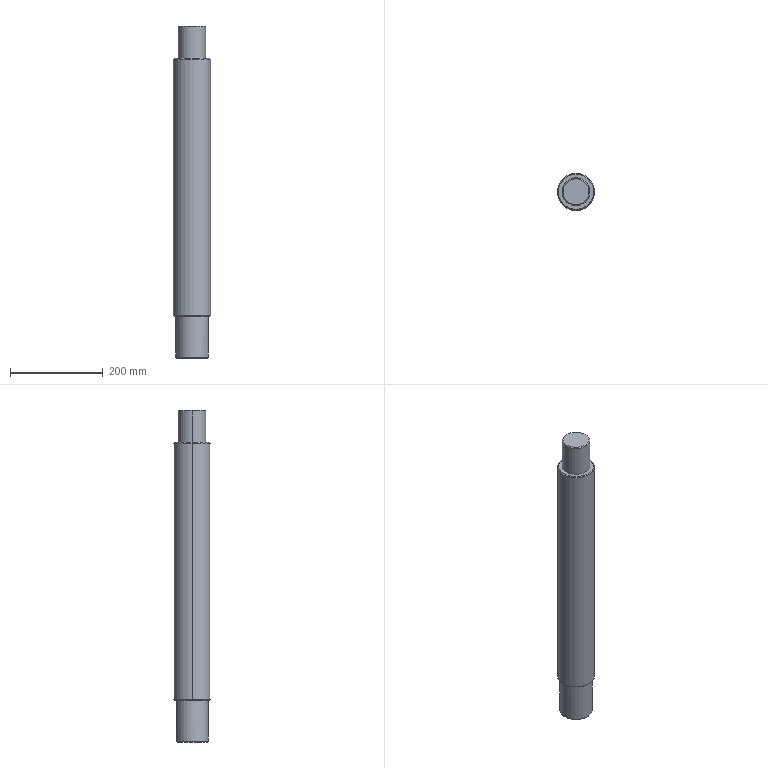Part | Creo | features CURVE 4, CUT 3, DATUM PLANE 3, CHAMFER 1, COORDINATE SYSTEM 1, PROTRUSION 1, ROUND 1 | 1 solid | 21 faces | box 80 x 80 x 717 mm | volume 3328283 mm3 | plane 7 | cylinder 7 | cone 7 | commonest cylinder face diameters 60 x2 70 x2 80 x2 20 x1
STEP:
#1=CARTESIAN_POINT('',(0.,0.,0.));
#2=DIRECTION('',(0.,0.,1.));
#3=DIRECTION('',(1.,0.,0.));
#4=AXIS2_PLACEMENT_3D('',#1,#2,#3);
#5=CARTESIAN_POINT('',(10.,31.448,0.));
#6=VERTEX_POINT('',#5);
#7=CARTESIAN_POINT('',(10.,26.541,0.));
#8=VERTEX_POINT('',#7);
#9=CARTESIAN_POINT('',(10.,31.448,0.));
#10=DIRECTION('',(0.,-1.,0.));
#11=VECTOR('',#10,4.907);
#12=LINE('',#9,#11);
#13=EDGE_CURVE('',#6,#8,#12,.T.);
#14=ORIENTED_EDGE('',*,*,#13,.T.);
#15=CARTESIAN_POINT('',(-10.,26.541,0.));
#16=VERTEX_POINT('',#15);
#17=CARTESIAN_POINT('',(10.,26.541,0.));
#18=DIRECTION('',(-1.,0.,0.));
#19=VECTOR('',#18,20.);
#20=LINE('',#17,#19);
#21=EDGE_CURVE('',#8,#16,#20,.T.);
#22=ORIENTED_EDGE('',*,*,#21,.T.);
#23=CARTESIAN_POINT('',(-10.,31.448,0.));
#24=VERTEX_POINT('',#23);
#25=CARTESIAN_POINT('',(-10.,31.448,0.));
#26=DIRECTION('',(0.,-1.,0.));
#27=VECTOR('',#26,4.907);
#28=LINE('',#25,#27);
#29=EDGE_CURVE('',#24,#16,#28,.T.);
#30=ORIENTED_EDGE('',*,*,#29,.F.);
#31=CARTESIAN_POINT('',(0.,0.,0.));
#32=DIRECTION('',(0.,0.,-1.));
#33=DIRECTION('',(0.303,0.953,0.));
#34=AXIS2_PLACEMENT_3D('',#31,#32,#33);
#35=CIRCLE('',#34,33.);
#36=EDGE_CURVE('',#6,#24,#35,.T.);
#37=ORIENTED_EDGE('',*,*,#36,.F.);
#38=EDGE_LOOP('',(#14,#22,#30,#37));
#39=FACE_OUTER_BOUND('',#38,.F.);
#40=CARTESIAN_POINT('',(0.,0.,0.));
#41=DIRECTION('',(0.,0.,1.));
#42=DIRECTION('',(1.,0.,0.));
#43=AXIS2_PLACEMENT_3D('',#40,#41,#42);
#44=PLANE('',#43);
#45=ADVANCED_FACE('',(#39),#44,.F.);
#46=CARTESIAN_POINT('',(10.,26.541,80.));
#47=VERTEX_POINT('',#46);
#48=CARTESIAN_POINT('',(10.,33.541,80.));
#49=VERTEX_POINT('',#48);
#50=CARTESIAN_POINT('',(10.,26.541,80.));
#51=DIRECTION('',(0.,1.,0.));
#52=VECTOR('',#51,7.);
#53=LINE('',#50,#52);
#54=EDGE_CURVE('',#47,#49,#53,.T.);
#55=ORIENTED_EDGE('',*,*,#54,.F.);
#56=CARTESIAN_POINT('',(10.,26.541,0.));
#57=DIRECTION('',(0.,0.,1.));
#58=VECTOR('',#57,80.);
#59=LINE('',#56,#58);
#60=EDGE_CURVE('',#8,#47,#59,.T.);
#61=ORIENTED_EDGE('',*,*,#60,.F.);
#62=ORIENTED_EDGE('',*,*,#13,.F.);
#63=CARTESIAN_POINT('',(10.,33.541,2.));
#64=VERTEX_POINT('',#63);
#65=CARTESIAN_POINT('',(10.,31.448,0.));
#66=CARTESIAN_POINT('',(10.,31.678,0.2193));
#67=CARTESIAN_POINT('',(10.,32.14,0.6599));
#68=CARTESIAN_POINT('',(10.,32.838,1.327));
#69=CARTESIAN_POINT('',(10.,33.306,1.775));
#70=B_SPLINE_CURVE_WITH_KNOTS('',3,(#65,#66,#67,#68,#69,#63),.UNSPECIFIED.,.F.,.F.,(4,1,1,4),(0.,0.3333,0.6667,1.),.UNSPECIFIED.);
#71=EDGE_CURVE('',#6,#64,#70,.T.);
#72=ORIENTED_EDGE('',*,*,#71,.T.);
#73=CARTESIAN_POINT('',(10.,33.541,80.));
#74=DIRECTION('',(0.,0.,-1.));
#75=VECTOR('',#74,78.);
#76=LINE('',#73,#75);
#77=EDGE_CURVE('',#49,#64,#76,.T.);
#78=ORIENTED_EDGE('',*,*,#77,.F.);
#79=EDGE_LOOP('',(#55,#61,#62,#72,#78));
#80=FACE_OUTER_BOUND('',#79,.F.);
#81=CARTESIAN_POINT('',(10.,33.541,0.));
#82=DIRECTION('',(1.,0.,0.));
#83=DIRECTION('',(0.,-1.,0.));
#84=AXIS2_PLACEMENT_3D('',#81,#82,#83);
#85=PLANE('',#84);
#86=ADVANCED_FACE('',(#80),#85,.F.);
#87=CARTESIAN_POINT('',(-10.,33.541,80.));
#88=VERTEX_POINT('',#87);
#89=CARTESIAN_POINT('',(-10.,26.541,80.));
#90=VERTEX_POINT('',#89);
#91=CARTESIAN_POINT('',(-10.,33.541,80.));
#92=DIRECTION('',(0.,-1.,0.));
#93=VECTOR('',#92,7.);
#94=LINE('',#91,#93);
#95=EDGE_CURVE('',#88,#90,#94,.T.);
#96=ORIENTED_EDGE('',*,*,#95,.T.);
#97=CARTESIAN_POINT('',(0.,26.541,80.));
#98=DIRECTION('',(0.,-1.,0.));
#99=DIRECTION('',(1.,0.,0.));
#100=AXIS2_PLACEMENT_3D('',#97,#98,#99);
#101=CIRCLE('',#100,10.);
#102=EDGE_CURVE('',#47,#90,#101,.T.);
#103=ORIENTED_EDGE('',*,*,#102,.F.);
#104=ORIENTED_EDGE('',*,*,#54,.T.);
#105=CARTESIAN_POINT('',(0.,35.,90.));
#106=VERTEX_POINT('',#105);
#107=CARTESIAN_POINT('',(10.,33.541,80.));
#108=CARTESIAN_POINT('',(10.,33.541,80.659));
#109=CARTESIAN_POINT('',(9.87,33.58,81.974));
#110=CARTESIAN_POINT('',(9.292,33.747,83.866));
#111=CARTESIAN_POINT('',(8.363,33.992,85.599));
#112=CARTESIAN_POINT('',(7.117,34.278,87.115));
#113=CARTESIAN_POINT('',(5.601,34.562,88.361));
#114=CARTESIAN_POINT('',(3.867,34.802,89.292));
#115=CARTESIAN_POINT('',(1.974,34.962,89.87));
#116=CARTESIAN_POINT('',(0.6588,35.,90.));
#117=CARTESIAN_POINT('',(0.,35.,90.));
#118=B_SPLINE_CURVE_WITH_KNOTS('',3,(#107,#108,#109,#110,#111,#112,#113,#114,#115,#116,#117),.UNSPECIFIED.,.F.,.F.,(4,1,1,1,1,1,1,1,4),(0.,0.125,0.25,0.375,0.5,0.625,0.75,0.875,1.),.UNSPECIFIED.);
#119=EDGE_CURVE('',#49,#106,#118,.T.);
#120=ORIENTED_EDGE('',*,*,#119,.T.);
#121=CARTESIAN_POINT('',(0.,35.,90.));
#122=CARTESIAN_POINT('',(-0.6588,35.,90.));
#123=CARTESIAN_POINT('',(-1.974,34.962,89.87));
#124=CARTESIAN_POINT('',(-3.867,34.802,89.292));
#125=CARTESIAN_POINT('',(-5.601,34.562,88.361));
#126=CARTESIAN_POINT('',(-7.117,34.279,87.115));
#127=CARTESIAN_POINT('',(-8.362,33.993,85.599));
#128=CARTESIAN_POINT('',(-9.292,33.747,83.866));
#129=CARTESIAN_POINT('',(-9.87,33.58,81.974));
#130=CARTESIAN_POINT('',(-10.,33.541,80.659));
#131=CARTESIAN_POINT('',(-10.,33.541,80.));
#132=B_SPLINE_CURVE_WITH_KNOTS('',3,(#121,#122,#123,#124,#125,#126,#127,#128,#129,#130,#131),.UNSPECIFIED.,.F.,.F.,(4,1,1,1,1,1,1,1,4),(0.,0.125,0.25,0.375,0.5,0.625,0.75,0.875,1.),.UNSPECIFIED.);
#133=EDGE_CURVE('',#106,#88,#132,.T.);
#134=ORIENTED_EDGE('',*,*,#133,.T.);
#135=EDGE_LOOP('',(#96,#103,#104,#120,#134));
#136=FACE_OUTER_BOUND('',#135,.F.);
#137=CARTESIAN_POINT('',(0.,144.288,80.));
#138=DIRECTION('',(0.,-1.,0.));
#139=DIRECTION('',(0.,0.,1.));
#140=AXIS2_PLACEMENT_3D('',#137,#138,#139);
#141=CYLINDRICAL_SURFACE('',#140,10.);
#142=ADVANCED_FACE('',(#136),#141,.F.);
#143=ORIENTED_EDGE('',*,*,#95,.F.);
#144=CARTESIAN_POINT('',(-10.,33.541,2.));
#145=VERTEX_POINT('',#144);
#146=CARTESIAN_POINT('',(-10.,33.541,80.));
#147=DIRECTION('',(0.,0.,-1.));
#148=VECTOR('',#147,78.);
#149=LINE('',#146,#148);
#150=EDGE_CURVE('',#88,#145,#149,.T.);
#151=ORIENTED_EDGE('',*,*,#150,.T.);
#152=CARTESIAN_POINT('',(-10.,33.306,1.775));
#153=CARTESIAN_POINT('',(-10.,32.838,1.327));
#154=CARTESIAN_POINT('',(-10.,32.14,0.66));
#155=CARTESIAN_POINT('',(-10.,31.679,0.2193));
#156=CARTESIAN_POINT('',(-10.,31.448,0.));
#157=B_SPLINE_CURVE_WITH_KNOTS('',3,(#144,#152,#153,#154,#155,#156),.UNSPECIFIED.,.F.,.F.,(4,1,1,4),(0.,0.3333,0.6667,1.),.UNSPECIFIED.);
#158=EDGE_CURVE('',#145,#24,#157,.T.);
#159=ORIENTED_EDGE('',*,*,#158,.T.);
#160=ORIENTED_EDGE('',*,*,#29,.T.);
#161=CARTESIAN_POINT('',(-10.,26.541,0.));
#162=DIRECTION('',(0.,0.,1.));
#163=VECTOR('',#162,80.);
#164=LINE('',#161,#163);
#165=EDGE_CURVE('',#16,#90,#164,.T.);
#166=ORIENTED_EDGE('',*,*,#165,.T.);
#167=EDGE_LOOP('',(#143,#151,#159,#160,#166));
#168=FACE_OUTER_BOUND('',#167,.F.);
#169=CARTESIAN_POINT('',(-10.,26.541,0.));
#170=DIRECTION('',(-1.,0.,0.));
#171=DIRECTION('',(0.,1.,0.));
#172=AXIS2_PLACEMENT_3D('',#169,#170,#171);
#173=PLANE('',#172);
#174=ADVANCED_FACE('',(#168),#173,.F.);
#175=CARTESIAN_POINT('',(-10.,33.541,90.));
#176=VERTEX_POINT('',#175);
#177=CARTESIAN_POINT('',(0.,0.,90.));
#178=DIRECTION('',(0.,0.,1.));
#179=DIRECTION('',(-0.2857,0.9583,0.));
#180=AXIS2_PLACEMENT_3D('',#177,#178,#179);
#181=CIRCLE('',#180,35.);
#182=EDGE_CURVE('',#176,#106,#181,.T.);
#183=ORIENTED_EDGE('',*,*,#182,.T.);
#184=ORIENTED_EDGE('',*,*,#119,.F.);
#185=ORIENTED_EDGE('',*,*,#77,.T.);
#186=CARTESIAN_POINT('',(0.,0.,2.));
#187=DIRECTION('',(0.,0.,1.));
#188=DIRECTION('',(-0.2857,0.9583,0.));
#189=AXIS2_PLACEMENT_3D('',#186,#187,#188);
#190=CIRCLE('',#189,35.);
#191=EDGE_CURVE('',#145,#64,#190,.T.);
#192=ORIENTED_EDGE('',*,*,#191,.F.);
#193=ORIENTED_EDGE('',*,*,#150,.F.);
#194=CARTESIAN_POINT('',(-10.,33.541,90.));
#195=DIRECTION('',(0.,0.,-1.));
#196=VECTOR('',#195,10.);
#197=LINE('',#194,#196);
#198=EDGE_CURVE('',#176,#88,#197,.T.);
#199=ORIENTED_EDGE('',*,*,#198,.F.);
#200=EDGE_LOOP('',(#183,#184,#185,#192,#193,#199));
#201=FACE_OUTER_BOUND('',#200,.F.);
#202=CARTESIAN_POINT('',(0.,0.,0.));
#203=DIRECTION('',(0.,0.,-1.));
#204=DIRECTION('',(-1.,0.,0.));
#205=AXIS2_PLACEMENT_3D('',#202,#203,#204);
#206=CYLINDRICAL_SURFACE('',#205,35.);
#207=ADVANCED_FACE('',(#201),#206,.T.);
#208=CARTESIAN_POINT('',(-38.,0.,90.));
#209=VERTEX_POINT('',#208);
#210=CARTESIAN_POINT('',(38.,0.,90.));
#211=VERTEX_POINT('',#210);
#212=CARTESIAN_POINT('',(0.,0.,90.));
#213=DIRECTION('',(0.,0.,1.));
#214=DIRECTION('',(-1.,0.,0.));
#215=AXIS2_PLACEMENT_3D('',#212,#213,#214);
#216=CIRCLE('',#215,38.);
#217=EDGE_CURVE('',#209,#211,#216,.T.);
#218=ORIENTED_EDGE('',*,*,#217,.T.);
#219=CARTESIAN_POINT('',(0.,0.,90.));
#220=DIRECTION('',(0.,0.,1.));
#221=DIRECTION('',(1.,0.,0.));
#222=AXIS2_PLACEMENT_3D('',#219,#220,#221);
#223=CIRCLE('',#222,38.);
#224=EDGE_CURVE('',#211,#209,#223,.T.);
#225=ORIENTED_EDGE('',*,*,#224,.T.);
#226=EDGE_LOOP('',(#218,#225));
#227=FACE_OUTER_BOUND('',#226,.F.);
#228=ORIENTED_EDGE('',*,*,#182,.F.);
#229=CARTESIAN_POINT('',(0.,0.,90.));
#230=DIRECTION('',(0.,0.,1.));
#231=DIRECTION('',(0.,1.,0.));
#232=AXIS2_PLACEMENT_3D('',#229,#230,#231);
#233=CIRCLE('',#232,35.);
#234=EDGE_CURVE('',#106,#176,#233,.T.);
#235=ORIENTED_EDGE('',*,*,#234,.F.);
#236=EDGE_LOOP('',(#228,#235));
#237=FACE_BOUND('',#236,.F.);
#238=CARTESIAN_POINT('',(0.,0.,90.));
#239=DIRECTION('',(0.,0.,-1.));
#240=DIRECTION('',(-1.,0.,0.));
#241=AXIS2_PLACEMENT_3D('',#238,#239,#240);
#242=PLANE('',#241);
#243=ADVANCED_FACE('',(#227,#237),#242,.T.);
#244=CARTESIAN_POINT('',(-40.,0.,92.));
#245=VERTEX_POINT('',#244);
#246=CARTESIAN_POINT('',(40.,0.,92.));
#247=VERTEX_POINT('',#246);
#248=CARTESIAN_POINT('',(0.,0.,92.));
#249=DIRECTION('',(0.,0.,1.));
#250=DIRECTION('',(-1.,0.,0.));
#251=AXIS2_PLACEMENT_3D('',#248,#249,#250);
#252=CIRCLE('',#251,40.);
#253=EDGE_CURVE('',#245,#247,#252,.T.);
#254=ORIENTED_EDGE('',*,*,#253,.T.);
#255=CARTESIAN_POINT('',(40.,0.000000005,92.));
#256=DIRECTION('',(-0.7071,0.,-0.7071));
#257=VECTOR('',#256,2.828);
#258=LINE('',#255,#257);
#259=EDGE_CURVE('',#247,#211,#258,.T.);
#260=ORIENTED_EDGE('',*,*,#259,.T.);
#261=ORIENTED_EDGE('',*,*,#217,.F.);
#262=CARTESIAN_POINT('',(-40.,-0.000000005,92.));
#263=DIRECTION('',(0.7071,0.,-0.7071));
#264=VECTOR('',#263,2.828);
#265=LINE('',#262,#264);
#266=EDGE_CURVE('',#245,#209,#265,.T.);
#267=ORIENTED_EDGE('',*,*,#266,.F.);
#268=EDGE_LOOP('',(#254,#260,#261,#267));
#269=FACE_OUTER_BOUND('',#268,.F.);
#270=CARTESIAN_POINT('',(0.,0.,91.));
#271=DIRECTION('',(0.,0.,1.));
#272=DIRECTION('',(0.,-1.,0.));
#273=AXIS2_PLACEMENT_3D('',#270,#271,#272);
#274=CONICAL_SURFACE('',#273,39.,45.);
#275=ADVANCED_FACE('',(#269),#274,.T.);
#276=CARTESIAN_POINT('',(40.,0.,645.));
#277=VERTEX_POINT('',#276);
#278=CARTESIAN_POINT('',(-40.,0.,645.));
#279=VERTEX_POINT('',#278);
#280=CARTESIAN_POINT('',(0.,0.,645.));
#281=DIRECTION('',(0.,0.,-1.));
#282=DIRECTION('',(1.,0.,0.));
#283=AXIS2_PLACEMENT_3D('',#280,#281,#282);
#284=CIRCLE('',#283,40.);
#285=EDGE_CURVE('',#277,#279,#284,.T.);
#286=ORIENTED_EDGE('',*,*,#285,.F.);
#287=CARTESIAN_POINT('',(40.,0.000000005,92.));
#288=DIRECTION('',(0.,0.,1.));
#289=VECTOR('',#288,553.);
#290=LINE('',#287,#289);
#291=EDGE_CURVE('',#247,#277,#290,.T.);
#292=ORIENTED_EDGE('',*,*,#291,.F.);
#293=ORIENTED_EDGE('',*,*,#253,.F.);
#294=CARTESIAN_POINT('',(-40.,-0.000000005,92.));
#295=DIRECTION('',(0.,0.,1.));
#296=VECTOR('',#295,553.);
#297=LINE('',#294,#296);
#298=EDGE_CURVE('',#245,#279,#297,.T.);
#299=ORIENTED_EDGE('',*,*,#298,.T.);
#300=EDGE_LOOP('',(#286,#292,#293,#299));
#301=FACE_OUTER_BOUND('',#300,.F.);
#302=CARTESIAN_POINT('',(0.,0.,0.));
#303=DIRECTION('',(0.,0.,1.));
#304=DIRECTION('',(1.,0.,0.));
#305=AXIS2_PLACEMENT_3D('',#302,#303,#304);
#306=CYLINDRICAL_SURFACE('',#305,40.);
#307=ADVANCED_FACE('',(#301),#306,.T.);
#308=ORIENTED_EDGE('',*,*,#285,.T.);
#309=CARTESIAN_POINT('',(-38.,0.,647.));
#310=VERTEX_POINT('',#309);
#311=CARTESIAN_POINT('',(-40.,-0.000000005,645.));
#312=DIRECTION('',(0.7071,0.,0.7071));
#313=VECTOR('',#312,2.828);
#314=LINE('',#311,#313);
#315=EDGE_CURVE('',#279,#310,#314,.T.);
#316=ORIENTED_EDGE('',*,*,#315,.T.);
#317=CARTESIAN_POINT('',(38.,0.,647.));
#318=VERTEX_POINT('',#317);
#319=CARTESIAN_POINT('',(0.,0.,647.));
#320=DIRECTION('',(0.,0.,-1.));
#321=DIRECTION('',(1.,0.,0.));
#322=AXIS2_PLACEMENT_3D('',#319,#320,#321);
#323=CIRCLE('',#322,38.);
#324=EDGE_CURVE('',#318,#310,#323,.T.);
#325=ORIENTED_EDGE('',*,*,#324,.F.);
#326=CARTESIAN_POINT('',(40.,0.000000005,645.));
#327=DIRECTION('',(-0.7071,0.,0.7071));
#328=VECTOR('',#327,2.828);
#329=LINE('',#326,#328);
#330=EDGE_CURVE('',#277,#318,#329,.T.);
#331=ORIENTED_EDGE('',*,*,#330,.F.);
#332=EDGE_LOOP('',(#308,#316,#325,#331));
#333=FACE_OUTER_BOUND('',#332,.F.);
#334=CARTESIAN_POINT('',(0.,0.,646.));
#335=DIRECTION('',(0.,0.,-1.));
#336=DIRECTION('',(0.,-1.,0.));
#337=AXIS2_PLACEMENT_3D('',#334,#335,#336);
#338=CONICAL_SURFACE('',#337,39.,45.);
#339=ADVANCED_FACE('',(#333),#338,.T.);
#340=CARTESIAN_POINT('',(0.,0.,645.));
#341=DIRECTION('',(0.,0.,-1.));
#342=DIRECTION('',(-1.,0.,0.));
#343=AXIS2_PLACEMENT_3D('',#340,#341,#342);
#344=CIRCLE('',#343,40.);
#345=EDGE_CURVE('',#279,#277,#344,.T.);
#346=ORIENTED_EDGE('',*,*,#345,.T.);
#347=ORIENTED_EDGE('',*,*,#330,.T.);
#348=CARTESIAN_POINT('',(0.,0.,647.));
#349=DIRECTION('',(0.,0.,-1.));
#350=DIRECTION('',(-1.,0.,0.));
#351=AXIS2_PLACEMENT_3D('',#348,#349,#350);
#352=CIRCLE('',#351,38.);
#353=EDGE_CURVE('',#310,#318,#352,.T.);
#354=ORIENTED_EDGE('',*,*,#353,.F.);
#355=ORIENTED_EDGE('',*,*,#315,.F.);
#356=EDGE_LOOP('',(#346,#347,#354,#355));
#357=FACE_OUTER_BOUND('',#356,.F.);
#358=CARTESIAN_POINT('',(0.,0.,646.));
#359=DIRECTION('',(0.,0.,-1.));
#360=DIRECTION('',(0.,-1.,0.));
#361=AXIS2_PLACEMENT_3D('',#358,#359,#360);
#362=CONICAL_SURFACE('',#361,39.,45.);
#363=ADVANCED_FACE('',(#357),#362,.T.);
#364=ORIENTED_EDGE('',*,*,#345,.F.);
#365=ORIENTED_EDGE('',*,*,#298,.F.);
#366=CARTESIAN_POINT('',(0.,0.,92.));
#367=DIRECTION('',(0.,0.,1.));
#368=DIRECTION('',(1.,0.,0.));
#369=AXIS2_PLACEMENT_3D('',#366,#367,#368);
#370=CIRCLE('',#369,40.);
#371=EDGE_CURVE('',#247,#245,#370,.T.);
#372=ORIENTED_EDGE('',*,*,#371,.F.);
#373=ORIENTED_EDGE('',*,*,#291,.T.);
#374=EDGE_LOOP('',(#364,#365,#372,#373));
#375=FACE_OUTER_BOUND('',#374,.F.);
#376=CARTESIAN_POINT('',(0.,0.,0.));
#377=DIRECTION('',(0.,0.,1.));
#378=DIRECTION('',(1.,0.,0.));
#379=AXIS2_PLACEMENT_3D('',#376,#377,#378);
#380=CYLINDRICAL_SURFACE('',#379,40.);
#381=ADVANCED_FACE('',(#375),#380,.T.);
#382=ORIENTED_EDGE('',*,*,#371,.T.);
#383=ORIENTED_EDGE('',*,*,#266,.T.);
#384=ORIENTED_EDGE('',*,*,#224,.F.);
#385=ORIENTED_EDGE('',*,*,#259,.F.);
#386=EDGE_LOOP('',(#382,#383,#384,#385));
#387=FACE_OUTER_BOUND('',#386,.F.);
#388=CARTESIAN_POINT('',(0.,0.,91.));
#389=DIRECTION('',(0.,0.,1.));
#390=DIRECTION('',(0.,-1.,0.));
#391=AXIS2_PLACEMENT_3D('',#388,#389,#390);
#392=CONICAL_SURFACE('',#391,39.,45.);
#393=ADVANCED_FACE('',(#387),#392,.T.);
#394=ORIENTED_EDGE('',*,*,#324,.T.);
#395=ORIENTED_EDGE('',*,*,#353,.T.);
#396=EDGE_LOOP('',(#394,#395));
#397=FACE_OUTER_BOUND('',#396,.F.);
#398=CARTESIAN_POINT('',(30.,0.,647.));
#399=VERTEX_POINT('',#398);
#400=CARTESIAN_POINT('',(-30.,0.,647.));
#401=VERTEX_POINT('',#400);
#402=CARTESIAN_POINT('',(0.,0.,647.));
#403=DIRECTION('',(0.,0.,-1.));
#404=DIRECTION('',(1.,0.,0.));
#405=AXIS2_PLACEMENT_3D('',#402,#403,#404);
#406=CIRCLE('',#405,30.);
#407=EDGE_CURVE('',#399,#401,#406,.T.);
#408=ORIENTED_EDGE('',*,*,#407,.F.);
#409=CARTESIAN_POINT('',(0.,0.,647.));
#410=DIRECTION('',(0.,0.,-1.));
#411=DIRECTION('',(-1.,0.,0.));
#412=AXIS2_PLACEMENT_3D('',#409,#410,#411);
#413=CIRCLE('',#412,30.);
#414=EDGE_CURVE('',#401,#399,#413,.T.);
#415=ORIENTED_EDGE('',*,*,#414,.F.);
#416=EDGE_LOOP('',(#408,#415));
#417=FACE_BOUND('',#416,.F.);
#418=CARTESIAN_POINT('',(0.,0.,647.));
#419=DIRECTION('',(0.,0.,1.));
#420=DIRECTION('',(1.,0.,0.));
#421=AXIS2_PLACEMENT_3D('',#418,#419,#420);
#422=PLANE('',#421);
#423=ADVANCED_FACE('',(#397,#417),#422,.T.);
#424=CARTESIAN_POINT('',(-30.,0.,715.));
#425=VERTEX_POINT('',#424);
#426=CARTESIAN_POINT('',(30.,0.,715.));
#427=VERTEX_POINT('',#426);
#428=CARTESIAN_POINT('',(0.,0.,715.));
#429=DIRECTION('',(0.,0.,1.));
#430=DIRECTION('',(-1.,0.,0.));
#431=AXIS2_PLACEMENT_3D('',#428,#429,#430);
#432=CIRCLE('',#431,30.);
#433=EDGE_CURVE('',#425,#427,#432,.T.);
#434=ORIENTED_EDGE('',*,*,#433,.T.);
#435=CARTESIAN_POINT('',(30.,-0.00000018,715.));
#436=DIRECTION('',(0.000000001,0.000000003,-1.));
#437=VECTOR('',#436,68.);
#438=LINE('',#435,#437);
#439=EDGE_CURVE('',#427,#399,#438,.T.);
#440=ORIENTED_EDGE('',*,*,#439,.T.);
#441=ORIENTED_EDGE('',*,*,#407,.T.);
#442=CARTESIAN_POINT('',(-30.,0.00000018,715.));
#443=DIRECTION('',(-0.000000001,-0.000000003,-1.));
#444=VECTOR('',#443,68.);
#445=LINE('',#442,#444);
#446=EDGE_CURVE('',#425,#401,#445,.T.);
#447=ORIENTED_EDGE('',*,*,#446,.F.);
#448=EDGE_LOOP('',(#434,#440,#441,#447));
#449=FACE_OUTER_BOUND('',#448,.F.);
#450=CARTESIAN_POINT('',(0.,0.,717.));
#451=DIRECTION('',(0.,0.,1.));
#452=DIRECTION('',(1.,0.,0.));
#453=AXIS2_PLACEMENT_3D('',#450,#451,#452);
#454=CYLINDRICAL_SURFACE('',#453,30.);
#455=ADVANCED_FACE('',(#449),#454,.T.);
#456=CARTESIAN_POINT('',(-28.,0.,717.));
#457=VERTEX_POINT('',#456);
#458=CARTESIAN_POINT('',(28.,0.,717.));
#459=VERTEX_POINT('',#458);
#460=CARTESIAN_POINT('',(0.,0.,717.));
#461=DIRECTION('',(0.,0.,1.));
#462=DIRECTION('',(-1.,0.,0.));
#463=AXIS2_PLACEMENT_3D('',#460,#461,#462);
#464=CIRCLE('',#463,28.);
#465=EDGE_CURVE('',#457,#459,#464,.T.);
#466=ORIENTED_EDGE('',*,*,#465,.T.);
#467=CARTESIAN_POINT('',(28.,-0.000000223,717.));
#468=DIRECTION('',(0.7071,0.000000016,-0.7071));
#469=VECTOR('',#468,2.828);
#470=LINE('',#467,#469);
#471=EDGE_CURVE('',#459,#427,#470,.T.);
#472=ORIENTED_EDGE('',*,*,#471,.T.);
#473=ORIENTED_EDGE('',*,*,#433,.F.);
#474=CARTESIAN_POINT('',(-28.,0.000000223,717.));
#475=DIRECTION('',(-0.7071,-0.000000016,-0.7071));
#476=VECTOR('',#475,2.828);
#477=LINE('',#474,#476);
#478=EDGE_CURVE('',#457,#425,#477,.T.);
#479=ORIENTED_EDGE('',*,*,#478,.F.);
#480=EDGE_LOOP('',(#466,#472,#473,#479));
#481=FACE_OUTER_BOUND('',#480,.F.);
#482=CARTESIAN_POINT('',(0.,0.,716.));
#483=DIRECTION('',(0.,0.,-1.));
#484=DIRECTION('',(0.,-1.,0.));
#485=AXIS2_PLACEMENT_3D('',#482,#483,#484);
#486=CONICAL_SURFACE('',#485,29.,45.);
#487=ADVANCED_FACE('',(#481),#486,.T.);
#488=ORIENTED_EDGE('',*,*,#465,.F.);
#489=CARTESIAN_POINT('',(0.,0.,717.));
#490=DIRECTION('',(0.,0.,1.));
#491=DIRECTION('',(1.,0.,0.));
#492=AXIS2_PLACEMENT_3D('',#489,#490,#491);
#493=CIRCLE('',#492,28.);
#494=EDGE_CURVE('',#459,#457,#493,.T.);
#495=ORIENTED_EDGE('',*,*,#494,.F.);
#496=EDGE_LOOP('',(#488,#495));
#497=FACE_OUTER_BOUND('',#496,.F.);
#498=CARTESIAN_POINT('',(0.,0.,717.));
#499=DIRECTION('',(0.,0.,1.));
#500=DIRECTION('',(1.,0.,0.));
#501=AXIS2_PLACEMENT_3D('',#498,#499,#500);
#502=PLANE('',#501);
#503=ADVANCED_FACE('',(#497),#502,.T.);
#504=ORIENTED_EDGE('',*,*,#494,.T.);
#505=ORIENTED_EDGE('',*,*,#478,.T.);
#506=CARTESIAN_POINT('',(0.,0.,715.));
#507=DIRECTION('',(0.,0.,1.));
#508=DIRECTION('',(1.,0.,0.));
#509=AXIS2_PLACEMENT_3D('',#506,#507,#508);
#510=CIRCLE('',#509,30.);
#511=EDGE_CURVE('',#427,#425,#510,.T.);
#512=ORIENTED_EDGE('',*,*,#511,.F.);
#513=ORIENTED_EDGE('',*,*,#471,.F.);
#514=EDGE_LOOP('',(#504,#505,#512,#513));
#515=FACE_OUTER_BOUND('',#514,.F.);
#516=CARTESIAN_POINT('',(0.,0.,716.));
#517=DIRECTION('',(0.,0.,-1.));
#518=DIRECTION('',(0.,-1.,0.));
#519=AXIS2_PLACEMENT_3D('',#516,#517,#518);
#520=CONICAL_SURFACE('',#519,29.,45.);
#521=ADVANCED_FACE('',(#515),#520,.T.);
#522=ORIENTED_EDGE('',*,*,#511,.T.);
#523=ORIENTED_EDGE('',*,*,#446,.T.);
#524=ORIENTED_EDGE('',*,*,#414,.T.);
#525=ORIENTED_EDGE('',*,*,#439,.F.);
#526=EDGE_LOOP('',(#522,#523,#524,#525));
#527=FACE_OUTER_BOUND('',#526,.F.);
#528=CARTESIAN_POINT('',(0.,0.,717.));
#529=DIRECTION('',(0.,0.,1.));
#530=DIRECTION('',(1.,0.,0.));
#531=AXIS2_PLACEMENT_3D('',#528,#529,#530);
#532=CYLINDRICAL_SURFACE('',#531,30.);
#533=ADVANCED_FACE('',(#527),#532,.T.);
#534=ORIENTED_EDGE('',*,*,#234,.T.);
#535=ORIENTED_EDGE('',*,*,#198,.T.);
#536=ORIENTED_EDGE('',*,*,#133,.F.);
#537=EDGE_LOOP('',(#534,#535,#536));
#538=FACE_OUTER_BOUND('',#537,.F.);
#539=CARTESIAN_POINT('',(0.,0.,0.));
#540=DIRECTION('',(0.,0.,-1.));
#541=DIRECTION('',(-1.,0.,0.));
#542=AXIS2_PLACEMENT_3D('',#539,#540,#541);
#543=CYLINDRICAL_SURFACE('',#542,35.);
#544=ADVANCED_FACE('',(#538),#543,.T.);
#545=ORIENTED_EDGE('',*,*,#36,.T.);
#546=ORIENTED_EDGE('',*,*,#158,.F.);
#547=ORIENTED_EDGE('',*,*,#191,.T.);
#548=ORIENTED_EDGE('',*,*,#71,.F.);
#549=EDGE_LOOP('',(#545,#546,#547,#548));
#550=FACE_OUTER_BOUND('',#549,.F.);
#551=CARTESIAN_POINT('',(0.,0.,1.));
#552=DIRECTION('',(0.,0.,1.));
#553=DIRECTION('',(0.,-1.,0.));
#554=AXIS2_PLACEMENT_3D('',#551,#552,#553);
#555=CONICAL_SURFACE('',#554,34.,45.);
#556=ADVANCED_FACE('',(#550),#555,.T.);
#557=ORIENTED_EDGE('',*,*,#102,.T.);
#558=ORIENTED_EDGE('',*,*,#165,.F.);
#559=ORIENTED_EDGE('',*,*,#21,.F.);
#560=ORIENTED_EDGE('',*,*,#60,.T.);
#561=EDGE_LOOP('',(#557,#558,#559,#560));
#562=FACE_OUTER_BOUND('',#561,.F.);
#563=CARTESIAN_POINT('',(10.,26.541,0.));
#564=DIRECTION('',(0.,-1.,0.));
#565=DIRECTION('',(-1.,0.,0.));
#566=AXIS2_PLACEMENT_3D('',#563,#564,#565);
#567=PLANE('',#566);
#568=ADVANCED_FACE('',(#562),#567,.F.);
#569=CLOSED_SHELL('',(#45,#86,#142,#174,#207,#243,#275,#307,#339,#363,#381,#393,#423,#455,#487,#503,#521,#533,#544,#556,#568));
#570=MANIFOLD_SOLID_BREP('',#569);
#571=(LENGTH_UNIT()NAMED_UNIT(*)SI_UNIT(.MILLI.,.METRE.));
#572=UNCERTAINTY_MEASURE_WITH_UNIT(LENGTH_MEASURE(0.07259),#571,'','');
#573=(NAMED_UNIT(*)PLANE_ANGLE_UNIT()SI_UNIT($,.RADIAN.));
#574=PLANE_ANGLE_MEASURE_WITH_UNIT(PLANE_ANGLE_MEASURE(0.01745),#573);
#575=(CONVERSION_BASED_UNIT('DEGREE',#574)NAMED_UNIT(*)PLANE_ANGLE_UNIT());
#576=(NAMED_UNIT(*)SI_UNIT($,.STERADIAN.)SOLID_ANGLE_UNIT());
#577=(GEOMETRIC_REPRESENTATION_CONTEXT(3)GLOBAL_UNCERTAINTY_ASSIGNED_CONTEXT((#572))GLOBAL_UNIT_ASSIGNED_CONTEXT((#571,#575,#576))REPRESENTATION_CONTEXT('',''));
#578=ADVANCED_BREP_SHAPE_REPRESENTATION('',(#4,#570),#577);